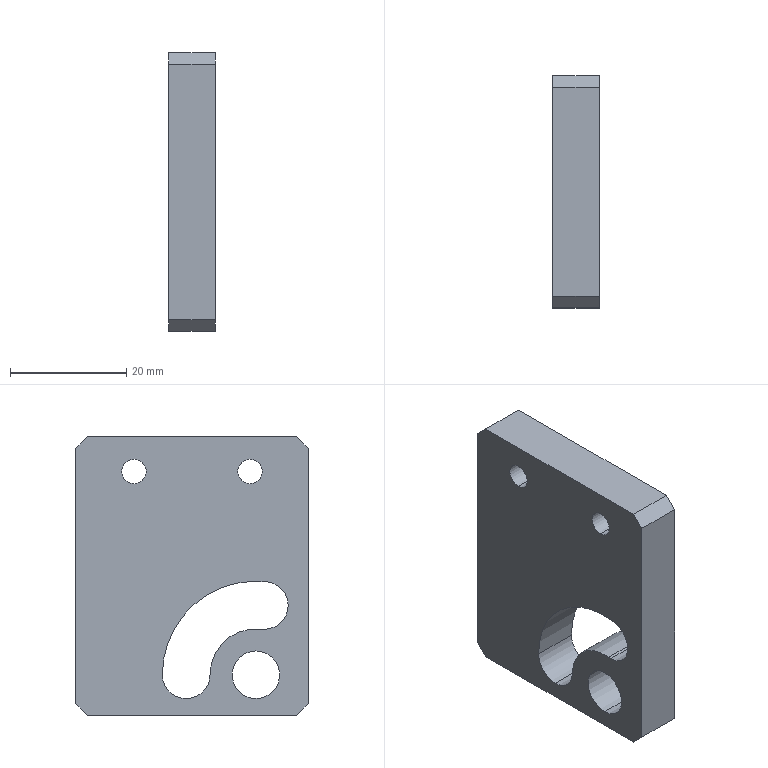Part | NX | features BREP 1 | 1 solid | 22 faces | box 8 x 40 x 48 mm | volume 12897 mm3 | cylinder 12 | plane 10 | commonest cylinder face diameters 8.2 x6 4.2 x4 15.8 x1 32.2 x1
STEP:
#1=CARTESIAN_POINT('',(8.,18.,-24.));
#2=VERTEX_POINT('',#1);
#3=CARTESIAN_POINT('',(8.,20.,-22.));
#4=VERTEX_POINT('',#3);
#5=CARTESIAN_POINT('',(8.,21.,-21.));
#6=DIRECTION('',(0.,0.7071,0.7071));
#7=VECTOR('',#6,1000.);
#8=LINE('',#5,#7);
#9=EDGE_CURVE('',#2,#4,#8,.T.);
#10=ORIENTED_EDGE('',*,*,#9,.F.);
#11=CARTESIAN_POINT('',(0.,18.,-24.));
#12=VERTEX_POINT('',#11);
#13=CARTESIAN_POINT('',(8.,18.,-24.));
#14=DIRECTION('',(1.,0.,0.));
#15=VECTOR('',#14,1000.);
#16=LINE('',#13,#15);
#17=EDGE_CURVE('',#12,#2,#16,.T.);
#18=ORIENTED_EDGE('',*,*,#17,.F.);
#19=CARTESIAN_POINT('',(0.,20.,-22.));
#20=VERTEX_POINT('',#19);
#21=CARTESIAN_POINT('',(0.,20.,-22.));
#22=DIRECTION('',(0.,-0.7071,-0.7071));
#23=VECTOR('',#22,1000.);
#24=LINE('',#21,#23);
#25=EDGE_CURVE('',#20,#12,#24,.T.);
#26=ORIENTED_EDGE('',*,*,#25,.F.);
#27=CARTESIAN_POINT('',(8.,20.,-22.));
#28=DIRECTION('',(-1.,0.,0.));
#29=VECTOR('',#28,1000.);
#30=LINE('',#27,#29);
#31=EDGE_CURVE('',#4,#20,#30,.T.);
#32=ORIENTED_EDGE('',*,*,#31,.F.);
#33=EDGE_LOOP('',(#10,#18,#26,#32));
#34=FACE_BOUND('',#33,.T.);
#35=CARTESIAN_POINT('',(8.,20.,-22.));
#36=DIRECTION('',(0.,-0.7071,0.7071));
#37=DIRECTION('',(-1.,0.,0.));
#38=AXIS2_PLACEMENT_3D('',#35,#36,#37);
#39=PLANE('',#38);
#40=ADVANCED_FACE('',(#34),#39,.F.);
#41=CARTESIAN_POINT('',(8.,-20.,-22.));
#42=VERTEX_POINT('',#41);
#43=CARTESIAN_POINT('',(8.,-18.,-24.));
#44=VERTEX_POINT('',#43);
#45=CARTESIAN_POINT('',(8.,-21.,-21.));
#46=DIRECTION('',(0.,0.7071,-0.7071));
#47=VECTOR('',#46,1000.);
#48=LINE('',#45,#47);
#49=EDGE_CURVE('',#42,#44,#48,.T.);
#50=ORIENTED_EDGE('',*,*,#49,.F.);
#51=CARTESIAN_POINT('',(0.,-20.,-22.));
#52=VERTEX_POINT('',#51);
#53=CARTESIAN_POINT('',(8.,-20.,-22.));
#54=DIRECTION('',(1.,0.,0.));
#55=VECTOR('',#54,1000.);
#56=LINE('',#53,#55);
#57=EDGE_CURVE('',#52,#42,#56,.T.);
#58=ORIENTED_EDGE('',*,*,#57,.F.);
#59=CARTESIAN_POINT('',(0.,-18.,-24.));
#60=VERTEX_POINT('',#59);
#61=CARTESIAN_POINT('',(0.,-18.,-24.));
#62=DIRECTION('',(0.,-0.7071,0.7071));
#63=VECTOR('',#62,1000.);
#64=LINE('',#61,#63);
#65=EDGE_CURVE('',#60,#52,#64,.T.);
#66=ORIENTED_EDGE('',*,*,#65,.F.);
#67=CARTESIAN_POINT('',(8.,-18.,-24.));
#68=DIRECTION('',(-1.,0.,0.));
#69=VECTOR('',#68,1000.);
#70=LINE('',#67,#69);
#71=EDGE_CURVE('',#44,#60,#70,.T.);
#72=ORIENTED_EDGE('',*,*,#71,.F.);
#73=EDGE_LOOP('',(#50,#58,#66,#72));
#74=FACE_BOUND('',#73,.T.);
#75=CARTESIAN_POINT('',(8.,-18.,-24.));
#76=DIRECTION('',(0.,0.7071,0.7071));
#77=DIRECTION('',(-1.,0.,0.));
#78=AXIS2_PLACEMENT_3D('',#75,#76,#77);
#79=PLANE('',#78);
#80=ADVANCED_FACE('',(#74),#79,.F.);
#81=CARTESIAN_POINT('',(8.,-18.,24.));
#82=VERTEX_POINT('',#81);
#83=CARTESIAN_POINT('',(8.,-20.,22.));
#84=VERTEX_POINT('',#83);
#85=CARTESIAN_POINT('',(8.,-21.,21.));
#86=DIRECTION('',(0.,-0.7071,-0.7071));
#87=VECTOR('',#86,1000.);
#88=LINE('',#85,#87);
#89=EDGE_CURVE('',#82,#84,#88,.T.);
#90=ORIENTED_EDGE('',*,*,#89,.F.);
#91=CARTESIAN_POINT('',(0.,-18.,24.));
#92=VERTEX_POINT('',#91);
#93=CARTESIAN_POINT('',(8.,-18.,24.));
#94=DIRECTION('',(1.,0.,0.));
#95=VECTOR('',#94,1000.);
#96=LINE('',#93,#95);
#97=EDGE_CURVE('',#92,#82,#96,.T.);
#98=ORIENTED_EDGE('',*,*,#97,.F.);
#99=CARTESIAN_POINT('',(0.,-20.,22.));
#100=VERTEX_POINT('',#99);
#101=CARTESIAN_POINT('',(0.,-20.,22.));
#102=DIRECTION('',(0.,0.7071,0.7071));
#103=VECTOR('',#102,1000.);
#104=LINE('',#101,#103);
#105=EDGE_CURVE('',#100,#92,#104,.T.);
#106=ORIENTED_EDGE('',*,*,#105,.F.);
#107=CARTESIAN_POINT('',(8.,-20.,22.));
#108=DIRECTION('',(-1.,0.,0.));
#109=VECTOR('',#108,1000.);
#110=LINE('',#107,#109);
#111=EDGE_CURVE('',#84,#100,#110,.T.);
#112=ORIENTED_EDGE('',*,*,#111,.F.);
#113=EDGE_LOOP('',(#90,#98,#106,#112));
#114=FACE_BOUND('',#113,.T.);
#115=CARTESIAN_POINT('',(8.,-20.,22.));
#116=DIRECTION('',(0.,0.7071,-0.7071));
#117=DIRECTION('',(-1.,0.,0.));
#118=AXIS2_PLACEMENT_3D('',#115,#116,#117);
#119=PLANE('',#118);
#120=ADVANCED_FACE('',(#114),#119,.F.);
#121=CARTESIAN_POINT('',(8.,20.,22.));
#122=VERTEX_POINT('',#121);
#123=CARTESIAN_POINT('',(8.,18.,24.));
#124=VERTEX_POINT('',#123);
#125=CARTESIAN_POINT('',(8.,21.,21.));
#126=DIRECTION('',(0.,-0.7071,0.7071));
#127=VECTOR('',#126,1000.);
#128=LINE('',#125,#127);
#129=EDGE_CURVE('',#122,#124,#128,.T.);
#130=ORIENTED_EDGE('',*,*,#129,.F.);
#131=CARTESIAN_POINT('',(0.,20.,22.));
#132=VERTEX_POINT('',#131);
#133=CARTESIAN_POINT('',(8.,20.,22.));
#134=DIRECTION('',(1.,0.,0.));
#135=VECTOR('',#134,1000.);
#136=LINE('',#133,#135);
#137=EDGE_CURVE('',#132,#122,#136,.T.);
#138=ORIENTED_EDGE('',*,*,#137,.F.);
#139=CARTESIAN_POINT('',(0.,18.,24.));
#140=VERTEX_POINT('',#139);
#141=CARTESIAN_POINT('',(0.,18.,24.));
#142=DIRECTION('',(0.,0.7071,-0.7071));
#143=VECTOR('',#142,1000.);
#144=LINE('',#141,#143);
#145=EDGE_CURVE('',#140,#132,#144,.T.);
#146=ORIENTED_EDGE('',*,*,#145,.F.);
#147=CARTESIAN_POINT('',(8.,18.,24.));
#148=DIRECTION('',(-1.,0.,0.));
#149=VECTOR('',#148,1000.);
#150=LINE('',#147,#149);
#151=EDGE_CURVE('',#124,#140,#150,.T.);
#152=ORIENTED_EDGE('',*,*,#151,.F.);
#153=EDGE_LOOP('',(#130,#138,#146,#152));
#154=FACE_BOUND('',#153,.T.);
#155=CARTESIAN_POINT('',(8.,18.,24.));
#156=DIRECTION('',(0.,-0.7071,-0.7071));
#157=DIRECTION('',(-1.,0.,0.));
#158=AXIS2_PLACEMENT_3D('',#155,#156,#157);
#159=PLANE('',#158);
#160=ADVANCED_FACE('',(#154),#159,.F.);
#161=CARTESIAN_POINT('',(0.,10.,20.1));
#162=VERTEX_POINT('',#161);
#163=CARTESIAN_POINT('',(8.,10.,20.1));
#164=VERTEX_POINT('',#163);
#165=CARTESIAN_POINT('',(8.,10.,20.1));
#166=DIRECTION('',(1.,0.,0.));
#167=VECTOR('',#166,1000.);
#168=LINE('',#165,#167);
#169=EDGE_CURVE('',#162,#164,#168,.T.);
#170=ORIENTED_EDGE('',*,*,#169,.F.);
#171=CARTESIAN_POINT('',(0.,10.,15.9));
#172=VERTEX_POINT('',#171);
#173=CARTESIAN_POINT('',(0.,10.,18.));
#174=DIRECTION('',(1.,0.,0.));
#175=DIRECTION('',(0.,0.,-1.));
#176=AXIS2_PLACEMENT_3D('',#173,#174,#175);
#177=CIRCLE('',#176,2.1);
#178=EDGE_CURVE('',#172,#162,#177,.T.);
#179=ORIENTED_EDGE('',*,*,#178,.F.);
#180=CARTESIAN_POINT('',(8.,10.,15.9));
#181=VERTEX_POINT('',#180);
#182=CARTESIAN_POINT('',(8.,10.,15.9));
#183=DIRECTION('',(1.,0.,0.));
#184=VECTOR('',#183,1000.);
#185=LINE('',#182,#184);
#186=EDGE_CURVE('',#172,#181,#185,.T.);
#187=ORIENTED_EDGE('',*,*,#186,.T.);
#188=CARTESIAN_POINT('',(8.,10.,18.));
#189=DIRECTION('',(1.,0.,0.));
#190=DIRECTION('',(0.,0.,-1.));
#191=AXIS2_PLACEMENT_3D('',#188,#189,#190);
#192=CIRCLE('',#191,2.1);
#193=EDGE_CURVE('',#181,#164,#192,.T.);
#194=ORIENTED_EDGE('',*,*,#193,.T.);
#195=EDGE_LOOP('',(#170,#179,#187,#194));
#196=FACE_BOUND('',#195,.T.);
#197=CARTESIAN_POINT('',(8.,10.,18.));
#198=DIRECTION('',(1.,0.,0.));
#199=DIRECTION('',(0.,0.,-1.));
#200=AXIS2_PLACEMENT_3D('',#197,#198,#199);
#201=CYLINDRICAL_SURFACE('',#200,2.1);
#202=ADVANCED_FACE('',(#196),#201,.F.);
#203=CARTESIAN_POINT('',(0.,-10.,20.1));
#204=VERTEX_POINT('',#203);
#205=CARTESIAN_POINT('',(8.,-10.,20.1));
#206=VERTEX_POINT('',#205);
#207=CARTESIAN_POINT('',(8.,-10.,20.1));
#208=DIRECTION('',(1.,0.,0.));
#209=VECTOR('',#208,1000.);
#210=LINE('',#207,#209);
#211=EDGE_CURVE('',#204,#206,#210,.T.);
#212=ORIENTED_EDGE('',*,*,#211,.F.);
#213=CARTESIAN_POINT('',(0.,-10.,15.9));
#214=VERTEX_POINT('',#213);
#215=CARTESIAN_POINT('',(0.,-10.,18.));
#216=DIRECTION('',(1.,0.,0.));
#217=DIRECTION('',(0.,0.,-1.));
#218=AXIS2_PLACEMENT_3D('',#215,#216,#217);
#219=CIRCLE('',#218,2.1);
#220=EDGE_CURVE('',#214,#204,#219,.T.);
#221=ORIENTED_EDGE('',*,*,#220,.F.);
#222=CARTESIAN_POINT('',(8.,-10.,15.9));
#223=VERTEX_POINT('',#222);
#224=CARTESIAN_POINT('',(8.,-10.,15.9));
#225=DIRECTION('',(1.,0.,0.));
#226=VECTOR('',#225,1000.);
#227=LINE('',#224,#226);
#228=EDGE_CURVE('',#214,#223,#227,.T.);
#229=ORIENTED_EDGE('',*,*,#228,.T.);
#230=CARTESIAN_POINT('',(8.,-10.,18.));
#231=DIRECTION('',(1.,0.,0.));
#232=DIRECTION('',(0.,0.,-1.));
#233=AXIS2_PLACEMENT_3D('',#230,#231,#232);
#234=CIRCLE('',#233,2.1);
#235=EDGE_CURVE('',#223,#206,#234,.T.);
#236=ORIENTED_EDGE('',*,*,#235,.T.);
#237=EDGE_LOOP('',(#212,#221,#229,#236));
#238=FACE_BOUND('',#237,.T.);
#239=CARTESIAN_POINT('',(8.,-10.,18.));
#240=DIRECTION('',(1.,0.,0.));
#241=DIRECTION('',(0.,0.,-1.));
#242=AXIS2_PLACEMENT_3D('',#239,#240,#241);
#243=CYLINDRICAL_SURFACE('',#242,2.1);
#244=ADVANCED_FACE('',(#238),#243,.F.);
#245=CARTESIAN_POINT('',(8.,5.1,-17.));
#246=VERTEX_POINT('',#245);
#247=CARTESIAN_POINT('',(8.,-12.962,-1.02));
#248=VERTEX_POINT('',#247);
#249=CARTESIAN_POINT('',(8.,-11.,-17.));
#250=DIRECTION('',(1.,0.,0.));
#251=DIRECTION('',(0.,0.,-1.));
#252=AXIS2_PLACEMENT_3D('',#249,#250,#251);
#253=CIRCLE('',#252,16.1);
#254=EDGE_CURVE('',#246,#248,#253,.T.);
#255=ORIENTED_EDGE('',*,*,#254,.T.);
#256=CARTESIAN_POINT('',(0.,-12.962,-1.02));
#257=VERTEX_POINT('',#256);
#258=CARTESIAN_POINT('',(0.,-12.962,-1.02));
#259=DIRECTION('',(1.,0.,0.));
#260=VECTOR('',#259,1000.);
#261=LINE('',#258,#260);
#262=EDGE_CURVE('',#257,#248,#261,.T.);
#263=ORIENTED_EDGE('',*,*,#262,.F.);
#264=CARTESIAN_POINT('',(0.,5.1,-17.));
#265=VERTEX_POINT('',#264);
#266=CARTESIAN_POINT('',(0.,-11.,-17.));
#267=DIRECTION('',(1.,0.,0.));
#268=DIRECTION('',(0.,0.,-1.));
#269=AXIS2_PLACEMENT_3D('',#266,#267,#268);
#270=CIRCLE('',#269,16.1);
#271=EDGE_CURVE('',#265,#257,#270,.T.);
#272=ORIENTED_EDGE('',*,*,#271,.F.);
#273=CARTESIAN_POINT('',(0.,5.1,-17.));
#274=DIRECTION('',(1.,0.,0.));
#275=VECTOR('',#274,1000.);
#276=LINE('',#273,#275);
#277=EDGE_CURVE('',#265,#246,#276,.T.);
#278=ORIENTED_EDGE('',*,*,#277,.T.);
#279=EDGE_LOOP('',(#255,#263,#272,#278));
#280=FACE_BOUND('',#279,.T.);
#281=CARTESIAN_POINT('',(0.,-11.,-17.));
#282=DIRECTION('',(1.,0.,0.));
#283=DIRECTION('',(0.,0.,-1.));
#284=AXIS2_PLACEMENT_3D('',#281,#282,#283);
#285=CYLINDRICAL_SURFACE('',#284,16.1);
#286=ADVANCED_FACE('',(#280),#285,.F.);
#287=CARTESIAN_POINT('',(0.,-12.462,-9.189));
#288=VERTEX_POINT('',#287);
#289=CARTESIAN_POINT('',(8.,-12.462,-9.189));
#290=VERTEX_POINT('',#289);
#291=CARTESIAN_POINT('',(0.,-12.462,-9.189));
#292=DIRECTION('',(1.,0.,0.));
#293=VECTOR('',#292,1000.);
#294=LINE('',#291,#293);
#295=EDGE_CURVE('',#288,#290,#294,.T.);
#296=ORIENTED_EDGE('',*,*,#295,.F.);
#297=CARTESIAN_POINT('',(0.,-12.462,-5.089));
#298=DIRECTION('',(1.,0.,0.));
#299=DIRECTION('',(0.,0.,-1.));
#300=AXIS2_PLACEMENT_3D('',#297,#298,#299);
#301=CIRCLE('',#300,4.1);
#302=EDGE_CURVE('',#257,#288,#301,.T.);
#303=ORIENTED_EDGE('',*,*,#302,.F.);
#304=ORIENTED_EDGE('',*,*,#262,.T.);
#305=CARTESIAN_POINT('',(8.,-12.462,-5.089));
#306=DIRECTION('',(1.,0.,0.));
#307=DIRECTION('',(0.,0.,-1.));
#308=AXIS2_PLACEMENT_3D('',#305,#306,#307);
#309=CIRCLE('',#308,4.1);
#310=EDGE_CURVE('',#248,#290,#309,.T.);
#311=ORIENTED_EDGE('',*,*,#310,.T.);
#312=EDGE_LOOP('',(#296,#303,#304,#311));
#313=FACE_BOUND('',#312,.T.);
#314=CARTESIAN_POINT('',(0.,-12.462,-5.089));
#315=DIRECTION('',(1.,0.,0.));
#316=DIRECTION('',(0.,0.,-1.));
#317=AXIS2_PLACEMENT_3D('',#314,#315,#316);
#318=CYLINDRICAL_SURFACE('',#317,4.1);
#319=ADVANCED_FACE('',(#313),#318,.F.);
#320=CARTESIAN_POINT('',(8.,-11.963,-9.159));
#321=VERTEX_POINT('',#320);
#322=CARTESIAN_POINT('',(8.,-3.1,-17.));
#323=VERTEX_POINT('',#322);
#324=CARTESIAN_POINT('',(8.,-11.,-17.));
#325=DIRECTION('',(-1.,0.,0.));
#326=DIRECTION('',(0.,0.,-1.));
#327=AXIS2_PLACEMENT_3D('',#324,#325,#326);
#328=CIRCLE('',#327,7.9);
#329=EDGE_CURVE('',#321,#323,#328,.T.);
#330=ORIENTED_EDGE('',*,*,#329,.T.);
#331=CARTESIAN_POINT('',(0.,-3.1,-17.));
#332=VERTEX_POINT('',#331);
#333=CARTESIAN_POINT('',(0.,-3.1,-17.));
#334=DIRECTION('',(1.,0.,0.));
#335=VECTOR('',#334,1000.);
#336=LINE('',#333,#335);
#337=EDGE_CURVE('',#332,#323,#336,.T.);
#338=ORIENTED_EDGE('',*,*,#337,.F.);
#339=CARTESIAN_POINT('',(0.,-11.963,-9.159));
#340=VERTEX_POINT('',#339);
#341=CARTESIAN_POINT('',(0.,-11.,-17.));
#342=DIRECTION('',(-1.,0.,0.));
#343=DIRECTION('',(0.,0.,-1.));
#344=AXIS2_PLACEMENT_3D('',#341,#342,#343);
#345=CIRCLE('',#344,7.9);
#346=EDGE_CURVE('',#340,#332,#345,.T.);
#347=ORIENTED_EDGE('',*,*,#346,.F.);
#348=CARTESIAN_POINT('',(0.,-11.963,-9.159));
#349=DIRECTION('',(1.,0.,0.));
#350=VECTOR('',#349,1000.);
#351=LINE('',#348,#350);
#352=EDGE_CURVE('',#340,#321,#351,.T.);
#353=ORIENTED_EDGE('',*,*,#352,.T.);
#354=EDGE_LOOP('',(#330,#338,#347,#353));
#355=FACE_BOUND('',#354,.T.);
#356=CARTESIAN_POINT('',(0.,-11.,-17.));
#357=DIRECTION('',(1.,0.,0.));
#358=DIRECTION('',(0.,0.,-1.));
#359=AXIS2_PLACEMENT_3D('',#356,#357,#358);
#360=CYLINDRICAL_SURFACE('',#359,7.9);
#361=ADVANCED_FACE('',(#355),#360,.T.);
#362=CARTESIAN_POINT('',(0.,1.,-21.1));
#363=VERTEX_POINT('',#362);
#364=CARTESIAN_POINT('',(8.,1.,-21.1));
#365=VERTEX_POINT('',#364);
#366=CARTESIAN_POINT('',(0.,1.,-21.1));
#367=DIRECTION('',(1.,0.,0.));
#368=VECTOR('',#367,1000.);
#369=LINE('',#366,#368);
#370=EDGE_CURVE('',#363,#365,#369,.T.);
#371=ORIENTED_EDGE('',*,*,#370,.F.);
#372=CARTESIAN_POINT('',(0.,1.,-17.));
#373=DIRECTION('',(1.,0.,0.));
#374=DIRECTION('',(0.,0.,-1.));
#375=AXIS2_PLACEMENT_3D('',#372,#373,#374);
#376=CIRCLE('',#375,4.1);
#377=EDGE_CURVE('',#332,#363,#376,.T.);
#378=ORIENTED_EDGE('',*,*,#377,.F.);
#379=ORIENTED_EDGE('',*,*,#337,.T.);
#380=CARTESIAN_POINT('',(8.,1.,-17.));
#381=DIRECTION('',(1.,0.,0.));
#382=DIRECTION('',(0.,0.,-1.));
#383=AXIS2_PLACEMENT_3D('',#380,#381,#382);
#384=CIRCLE('',#383,4.1);
#385=EDGE_CURVE('',#323,#365,#384,.T.);
#386=ORIENTED_EDGE('',*,*,#385,.T.);
#387=EDGE_LOOP('',(#371,#378,#379,#386));
#388=FACE_BOUND('',#387,.T.);
#389=CARTESIAN_POINT('',(0.,1.,-17.));
#390=DIRECTION('',(1.,0.,0.));
#391=DIRECTION('',(0.,0.,-1.));
#392=AXIS2_PLACEMENT_3D('',#389,#390,#391);
#393=CYLINDRICAL_SURFACE('',#392,4.1);
#394=ADVANCED_FACE('',(#388),#393,.F.);
#395=CARTESIAN_POINT('',(0.,-11.,-12.9));
#396=VERTEX_POINT('',#395);
#397=CARTESIAN_POINT('',(8.,-11.,-12.9));
#398=VERTEX_POINT('',#397);
#399=CARTESIAN_POINT('',(0.,-11.,-12.9));
#400=DIRECTION('',(1.,0.,0.));
#401=VECTOR('',#400,1000.);
#402=LINE('',#399,#401);
#403=EDGE_CURVE('',#396,#398,#402,.T.);
#404=ORIENTED_EDGE('',*,*,#403,.F.);
#405=CARTESIAN_POINT('',(0.,-11.,-21.1));
#406=VERTEX_POINT('',#405);
#407=CARTESIAN_POINT('',(0.,-11.,-17.));
#408=DIRECTION('',(1.,0.,0.));
#409=DIRECTION('',(0.,0.,-1.));
#410=AXIS2_PLACEMENT_3D('',#407,#408,#409);
#411=CIRCLE('',#410,4.1);
#412=EDGE_CURVE('',#406,#396,#411,.T.);
#413=ORIENTED_EDGE('',*,*,#412,.F.);
#414=CARTESIAN_POINT('',(8.,-11.,-21.1));
#415=VERTEX_POINT('',#414);
#416=CARTESIAN_POINT('',(0.,-11.,-21.1));
#417=DIRECTION('',(1.,0.,0.));
#418=VECTOR('',#417,1000.);
#419=LINE('',#416,#418);
#420=EDGE_CURVE('',#406,#415,#419,.T.);
#421=ORIENTED_EDGE('',*,*,#420,.T.);
#422=CARTESIAN_POINT('',(8.,-11.,-17.));
#423=DIRECTION('',(1.,0.,0.));
#424=DIRECTION('',(0.,0.,-1.));
#425=AXIS2_PLACEMENT_3D('',#422,#423,#424);
#426=CIRCLE('',#425,4.1);
#427=EDGE_CURVE('',#415,#398,#426,.T.);
#428=ORIENTED_EDGE('',*,*,#427,.T.);
#429=EDGE_LOOP('',(#404,#413,#421,#428));
#430=FACE_BOUND('',#429,.T.);
#431=CARTESIAN_POINT('',(0.,-11.,-17.));
#432=DIRECTION('',(1.,0.,0.));
#433=DIRECTION('',(0.,0.,-1.));
#434=AXIS2_PLACEMENT_3D('',#431,#432,#433);
#435=CYLINDRICAL_SURFACE('',#434,4.1);
#436=ADVANCED_FACE('',(#430),#435,.F.);
#437=CARTESIAN_POINT('',(0.,-20.,24.));
#438=DIRECTION('',(0.,-1.,0.));
#439=VECTOR('',#438,1000.);
#440=LINE('',#437,#439);
#441=EDGE_CURVE('',#140,#92,#440,.T.);
#442=ORIENTED_EDGE('',*,*,#441,.F.);
#443=ORIENTED_EDGE('',*,*,#145,.T.);
#444=CARTESIAN_POINT('',(0.,20.,-24.));
#445=DIRECTION('',(0.,0.,1.));
#446=VECTOR('',#445,1000.);
#447=LINE('',#444,#446);
#448=EDGE_CURVE('',#20,#132,#447,.T.);
#449=ORIENTED_EDGE('',*,*,#448,.F.);
#450=ORIENTED_EDGE('',*,*,#25,.T.);
#451=CARTESIAN_POINT('',(0.,-20.,-24.));
#452=DIRECTION('',(0.,1.,0.));
#453=VECTOR('',#452,1000.);
#454=LINE('',#451,#453);
#455=EDGE_CURVE('',#60,#12,#454,.T.);
#456=ORIENTED_EDGE('',*,*,#455,.F.);
#457=ORIENTED_EDGE('',*,*,#65,.T.);
#458=CARTESIAN_POINT('',(0.,-20.,-24.));
#459=DIRECTION('',(0.,0.,-1.));
#460=VECTOR('',#459,1000.);
#461=LINE('',#458,#460);
#462=EDGE_CURVE('',#100,#52,#461,.T.);
#463=ORIENTED_EDGE('',*,*,#462,.F.);
#464=ORIENTED_EDGE('',*,*,#105,.T.);
#465=EDGE_LOOP('',(#442,#443,#449,#450,#456,#457,#463,#464));
#466=FACE_BOUND('',#465,.T.);
#467=ORIENTED_EDGE('',*,*,#412,.T.);
#468=CARTESIAN_POINT('',(0.,-11.,-17.));
#469=DIRECTION('',(1.,0.,0.));
#470=DIRECTION('',(0.,0.,-1.));
#471=AXIS2_PLACEMENT_3D('',#468,#469,#470);
#472=CIRCLE('',#471,4.1);
#473=EDGE_CURVE('',#396,#406,#472,.T.);
#474=ORIENTED_EDGE('',*,*,#473,.T.);
#475=EDGE_LOOP('',(#467,#474));
#476=FACE_BOUND('',#475,.T.);
#477=ORIENTED_EDGE('',*,*,#346,.T.);
#478=ORIENTED_EDGE('',*,*,#377,.T.);
#479=CARTESIAN_POINT('',(0.,1.,-17.));
#480=DIRECTION('',(1.,0.,0.));
#481=DIRECTION('',(0.,0.,-1.));
#482=AXIS2_PLACEMENT_3D('',#479,#480,#481);
#483=CIRCLE('',#482,4.1);
#484=EDGE_CURVE('',#363,#265,#483,.T.);
#485=ORIENTED_EDGE('',*,*,#484,.T.);
#486=ORIENTED_EDGE('',*,*,#271,.T.);
#487=ORIENTED_EDGE('',*,*,#302,.T.);
#488=CARTESIAN_POINT('',(0.,-12.462,-5.089));
#489=DIRECTION('',(1.,0.,0.));
#490=DIRECTION('',(0.,0.,-1.));
#491=AXIS2_PLACEMENT_3D('',#488,#489,#490);
#492=CIRCLE('',#491,4.1);
#493=EDGE_CURVE('',#288,#340,#492,.T.);
#494=ORIENTED_EDGE('',*,*,#493,.T.);
#495=EDGE_LOOP('',(#477,#478,#485,#486,#487,#494));
#496=FACE_BOUND('',#495,.T.);
#497=ORIENTED_EDGE('',*,*,#220,.T.);
#498=CARTESIAN_POINT('',(0.,-10.,18.));
#499=DIRECTION('',(1.,0.,0.));
#500=DIRECTION('',(0.,0.,-1.));
#501=AXIS2_PLACEMENT_3D('',#498,#499,#500);
#502=CIRCLE('',#501,2.1);
#503=EDGE_CURVE('',#204,#214,#502,.T.);
#504=ORIENTED_EDGE('',*,*,#503,.T.);
#505=EDGE_LOOP('',(#497,#504));
#506=FACE_BOUND('',#505,.T.);
#507=ORIENTED_EDGE('',*,*,#178,.T.);
#508=CARTESIAN_POINT('',(0.,10.,18.));
#509=DIRECTION('',(1.,0.,0.));
#510=DIRECTION('',(0.,0.,-1.));
#511=AXIS2_PLACEMENT_3D('',#508,#509,#510);
#512=CIRCLE('',#511,2.1);
#513=EDGE_CURVE('',#162,#172,#512,.T.);
#514=ORIENTED_EDGE('',*,*,#513,.T.);
#515=EDGE_LOOP('',(#507,#514));
#516=FACE_BOUND('',#515,.T.);
#517=CARTESIAN_POINT('',(0.,0.,0.));
#518=DIRECTION('',(1.,0.,0.));
#519=DIRECTION('',(0.,0.,-1.));
#520=AXIS2_PLACEMENT_3D('',#517,#518,#519);
#521=PLANE('',#520);
#522=ADVANCED_FACE('',(#466,#476,#496,#506,#516),#521,.F.);
#523=CARTESIAN_POINT('',(8.,20.,-24.));
#524=DIRECTION('',(0.,0.,1.));
#525=VECTOR('',#524,1000.);
#526=LINE('',#523,#525);
#527=EDGE_CURVE('',#4,#122,#526,.T.);
#528=ORIENTED_EDGE('',*,*,#527,.T.);
#529=ORIENTED_EDGE('',*,*,#129,.T.);
#530=CARTESIAN_POINT('',(8.,-20.,24.));
#531=DIRECTION('',(0.,-1.,0.));
#532=VECTOR('',#531,1000.);
#533=LINE('',#530,#532);
#534=EDGE_CURVE('',#124,#82,#533,.T.);
#535=ORIENTED_EDGE('',*,*,#534,.T.);
#536=ORIENTED_EDGE('',*,*,#89,.T.);
#537=CARTESIAN_POINT('',(8.,-20.,-24.));
#538=DIRECTION('',(0.,0.,-1.));
#539=VECTOR('',#538,1000.);
#540=LINE('',#537,#539);
#541=EDGE_CURVE('',#84,#42,#540,.T.);
#542=ORIENTED_EDGE('',*,*,#541,.T.);
#543=ORIENTED_EDGE('',*,*,#49,.T.);
#544=CARTESIAN_POINT('',(8.,-20.,-24.));
#545=DIRECTION('',(0.,1.,0.));
#546=VECTOR('',#545,1000.);
#547=LINE('',#544,#546);
#548=EDGE_CURVE('',#44,#2,#547,.T.);
#549=ORIENTED_EDGE('',*,*,#548,.T.);
#550=ORIENTED_EDGE('',*,*,#9,.T.);
#551=EDGE_LOOP('',(#528,#529,#535,#536,#542,#543,#549,#550));
#552=FACE_BOUND('',#551,.T.);
#553=ORIENTED_EDGE('',*,*,#427,.F.);
#554=CARTESIAN_POINT('',(8.,-11.,-17.));
#555=DIRECTION('',(1.,0.,0.));
#556=DIRECTION('',(0.,0.,-1.));
#557=AXIS2_PLACEMENT_3D('',#554,#555,#556);
#558=CIRCLE('',#557,4.1);
#559=EDGE_CURVE('',#398,#415,#558,.T.);
#560=ORIENTED_EDGE('',*,*,#559,.F.);
#561=EDGE_LOOP('',(#553,#560));
#562=FACE_BOUND('',#561,.T.);
#563=ORIENTED_EDGE('',*,*,#385,.F.);
#564=ORIENTED_EDGE('',*,*,#329,.F.);
#565=CARTESIAN_POINT('',(8.,-12.462,-5.089));
#566=DIRECTION('',(1.,0.,0.));
#567=DIRECTION('',(0.,0.,-1.));
#568=AXIS2_PLACEMENT_3D('',#565,#566,#567);
#569=CIRCLE('',#568,4.1);
#570=EDGE_CURVE('',#290,#321,#569,.T.);
#571=ORIENTED_EDGE('',*,*,#570,.F.);
#572=ORIENTED_EDGE('',*,*,#310,.F.);
#573=ORIENTED_EDGE('',*,*,#254,.F.);
#574=CARTESIAN_POINT('',(8.,1.,-17.));
#575=DIRECTION('',(1.,0.,0.));
#576=DIRECTION('',(0.,0.,-1.));
#577=AXIS2_PLACEMENT_3D('',#574,#575,#576);
#578=CIRCLE('',#577,4.1);
#579=EDGE_CURVE('',#365,#246,#578,.T.);
#580=ORIENTED_EDGE('',*,*,#579,.F.);
#581=EDGE_LOOP('',(#563,#564,#571,#572,#573,#580));
#582=FACE_BOUND('',#581,.T.);
#583=ORIENTED_EDGE('',*,*,#235,.F.);
#584=CARTESIAN_POINT('',(8.,-10.,18.));
#585=DIRECTION('',(1.,0.,0.));
#586=DIRECTION('',(0.,0.,-1.));
#587=AXIS2_PLACEMENT_3D('',#584,#585,#586);
#588=CIRCLE('',#587,2.1);
#589=EDGE_CURVE('',#206,#223,#588,.T.);
#590=ORIENTED_EDGE('',*,*,#589,.F.);
#591=EDGE_LOOP('',(#583,#590));
#592=FACE_BOUND('',#591,.T.);
#593=ORIENTED_EDGE('',*,*,#193,.F.);
#594=CARTESIAN_POINT('',(8.,10.,18.));
#595=DIRECTION('',(1.,0.,0.));
#596=DIRECTION('',(0.,0.,-1.));
#597=AXIS2_PLACEMENT_3D('',#594,#595,#596);
#598=CIRCLE('',#597,2.1);
#599=EDGE_CURVE('',#164,#181,#598,.T.);
#600=ORIENTED_EDGE('',*,*,#599,.F.);
#601=EDGE_LOOP('',(#593,#600));
#602=FACE_BOUND('',#601,.T.);
#603=CARTESIAN_POINT('',(8.,0.,0.));
#604=DIRECTION('',(1.,0.,0.));
#605=DIRECTION('',(0.,0.,-1.));
#606=AXIS2_PLACEMENT_3D('',#603,#604,#605);
#607=PLANE('',#606);
#608=ADVANCED_FACE('',(#552,#562,#582,#592,#602),#607,.T.);
#609=ORIENTED_EDGE('',*,*,#448,.T.);
#610=ORIENTED_EDGE('',*,*,#137,.T.);
#611=ORIENTED_EDGE('',*,*,#527,.F.);
#612=ORIENTED_EDGE('',*,*,#31,.T.);
#613=EDGE_LOOP('',(#609,#610,#611,#612));
#614=FACE_BOUND('',#613,.T.);
#615=CARTESIAN_POINT('',(8.,20.,-24.));
#616=DIRECTION('',(0.,-1.,0.));
#617=DIRECTION('',(0.,0.,-1.));
#618=AXIS2_PLACEMENT_3D('',#615,#616,#617);
#619=PLANE('',#618);
#620=ADVANCED_FACE('',(#614),#619,.F.);
#621=ORIENTED_EDGE('',*,*,#548,.F.);
#622=ORIENTED_EDGE('',*,*,#71,.T.);
#623=ORIENTED_EDGE('',*,*,#455,.T.);
#624=ORIENTED_EDGE('',*,*,#17,.T.);
#625=EDGE_LOOP('',(#621,#622,#623,#624));
#626=FACE_BOUND('',#625,.T.);
#627=CARTESIAN_POINT('',(8.,-20.,-24.));
#628=DIRECTION('',(0.,0.,1.));
#629=DIRECTION('',(1.,0.,0.));
#630=AXIS2_PLACEMENT_3D('',#627,#628,#629);
#631=PLANE('',#630);
#632=ADVANCED_FACE('',(#626),#631,.F.);
#633=ORIENTED_EDGE('',*,*,#541,.F.);
#634=ORIENTED_EDGE('',*,*,#111,.T.);
#635=ORIENTED_EDGE('',*,*,#462,.T.);
#636=ORIENTED_EDGE('',*,*,#57,.T.);
#637=EDGE_LOOP('',(#633,#634,#635,#636));
#638=FACE_BOUND('',#637,.T.);
#639=CARTESIAN_POINT('',(8.,-20.,-24.));
#640=DIRECTION('',(0.,1.,0.));
#641=DIRECTION('',(0.,0.,1.));
#642=AXIS2_PLACEMENT_3D('',#639,#640,#641);
#643=PLANE('',#642);
#644=ADVANCED_FACE('',(#638),#643,.F.);
#645=ORIENTED_EDGE('',*,*,#534,.F.);
#646=ORIENTED_EDGE('',*,*,#151,.T.);
#647=ORIENTED_EDGE('',*,*,#441,.T.);
#648=ORIENTED_EDGE('',*,*,#97,.T.);
#649=EDGE_LOOP('',(#645,#646,#647,#648));
#650=FACE_BOUND('',#649,.T.);
#651=CARTESIAN_POINT('',(8.,-20.,24.));
#652=DIRECTION('',(0.,0.,-1.));
#653=DIRECTION('',(-1.,0.,0.));
#654=AXIS2_PLACEMENT_3D('',#651,#652,#653);
#655=PLANE('',#654);
#656=ADVANCED_FACE('',(#650),#655,.F.);
#657=ORIENTED_EDGE('',*,*,#473,.F.);
#658=ORIENTED_EDGE('',*,*,#403,.T.);
#659=ORIENTED_EDGE('',*,*,#559,.T.);
#660=ORIENTED_EDGE('',*,*,#420,.F.);
#661=EDGE_LOOP('',(#657,#658,#659,#660));
#662=FACE_BOUND('',#661,.T.);
#663=CARTESIAN_POINT('',(0.,-11.,-17.));
#664=DIRECTION('',(1.,0.,0.));
#665=DIRECTION('',(0.,0.,-1.));
#666=AXIS2_PLACEMENT_3D('',#663,#664,#665);
#667=CYLINDRICAL_SURFACE('',#666,4.1);
#668=ADVANCED_FACE('',(#662),#667,.F.);
#669=ORIENTED_EDGE('',*,*,#484,.F.);
#670=ORIENTED_EDGE('',*,*,#370,.T.);
#671=ORIENTED_EDGE('',*,*,#579,.T.);
#672=ORIENTED_EDGE('',*,*,#277,.F.);
#673=EDGE_LOOP('',(#669,#670,#671,#672));
#674=FACE_BOUND('',#673,.T.);
#675=CARTESIAN_POINT('',(0.,1.,-17.));
#676=DIRECTION('',(1.,0.,0.));
#677=DIRECTION('',(0.,0.,-1.));
#678=AXIS2_PLACEMENT_3D('',#675,#676,#677);
#679=CYLINDRICAL_SURFACE('',#678,4.1);
#680=ADVANCED_FACE('',(#674),#679,.F.);
#681=ORIENTED_EDGE('',*,*,#493,.F.);
#682=ORIENTED_EDGE('',*,*,#295,.T.);
#683=ORIENTED_EDGE('',*,*,#570,.T.);
#684=ORIENTED_EDGE('',*,*,#352,.F.);
#685=EDGE_LOOP('',(#681,#682,#683,#684));
#686=FACE_BOUND('',#685,.T.);
#687=CARTESIAN_POINT('',(0.,-12.462,-5.089));
#688=DIRECTION('',(1.,0.,0.));
#689=DIRECTION('',(0.,0.,-1.));
#690=AXIS2_PLACEMENT_3D('',#687,#688,#689);
#691=CYLINDRICAL_SURFACE('',#690,4.1);
#692=ADVANCED_FACE('',(#686),#691,.F.);
#693=ORIENTED_EDGE('',*,*,#503,.F.);
#694=ORIENTED_EDGE('',*,*,#211,.T.);
#695=ORIENTED_EDGE('',*,*,#589,.T.);
#696=ORIENTED_EDGE('',*,*,#228,.F.);
#697=EDGE_LOOP('',(#693,#694,#695,#696));
#698=FACE_BOUND('',#697,.T.);
#699=CARTESIAN_POINT('',(8.,-10.,18.));
#700=DIRECTION('',(1.,0.,0.));
#701=DIRECTION('',(0.,0.,-1.));
#702=AXIS2_PLACEMENT_3D('',#699,#700,#701);
#703=CYLINDRICAL_SURFACE('',#702,2.1);
#704=ADVANCED_FACE('',(#698),#703,.F.);
#705=ORIENTED_EDGE('',*,*,#513,.F.);
#706=ORIENTED_EDGE('',*,*,#169,.T.);
#707=ORIENTED_EDGE('',*,*,#599,.T.);
#708=ORIENTED_EDGE('',*,*,#186,.F.);
#709=EDGE_LOOP('',(#705,#706,#707,#708));
#710=FACE_BOUND('',#709,.T.);
#711=CARTESIAN_POINT('',(8.,10.,18.));
#712=DIRECTION('',(1.,0.,0.));
#713=DIRECTION('',(0.,0.,-1.));
#714=AXIS2_PLACEMENT_3D('',#711,#712,#713);
#715=CYLINDRICAL_SURFACE('',#714,2.1);
#716=ADVANCED_FACE('',(#710),#715,.F.);
#717=CLOSED_SHELL('',(#40,#80,#120,#160,#202,#244,#286,#319,#361,#394,#436,#522,#608,#620,#632,#644,#656,#668,#680,#692,#704,#716));
#718=MANIFOLD_SOLID_BREP('',#717);
#719=(LENGTH_UNIT()NAMED_UNIT(*)SI_UNIT(.MILLI.,.METRE.));
#720=UNCERTAINTY_MEASURE_WITH_UNIT(LENGTH_MEASURE(0.00001),#719,'','');
#721=(NAMED_UNIT(*)PLANE_ANGLE_UNIT()SI_UNIT($,.RADIAN.));
#722=(NAMED_UNIT(*)SI_UNIT($,.STERADIAN.)SOLID_ANGLE_UNIT());
#723=(GEOMETRIC_REPRESENTATION_CONTEXT(3)GLOBAL_UNCERTAINTY_ASSIGNED_CONTEXT((#720))GLOBAL_UNIT_ASSIGNED_CONTEXT((#719,#721,#722))REPRESENTATION_CONTEXT('',''));
#724=ADVANCED_BREP_SHAPE_REPRESENTATION('',(#718),#723);